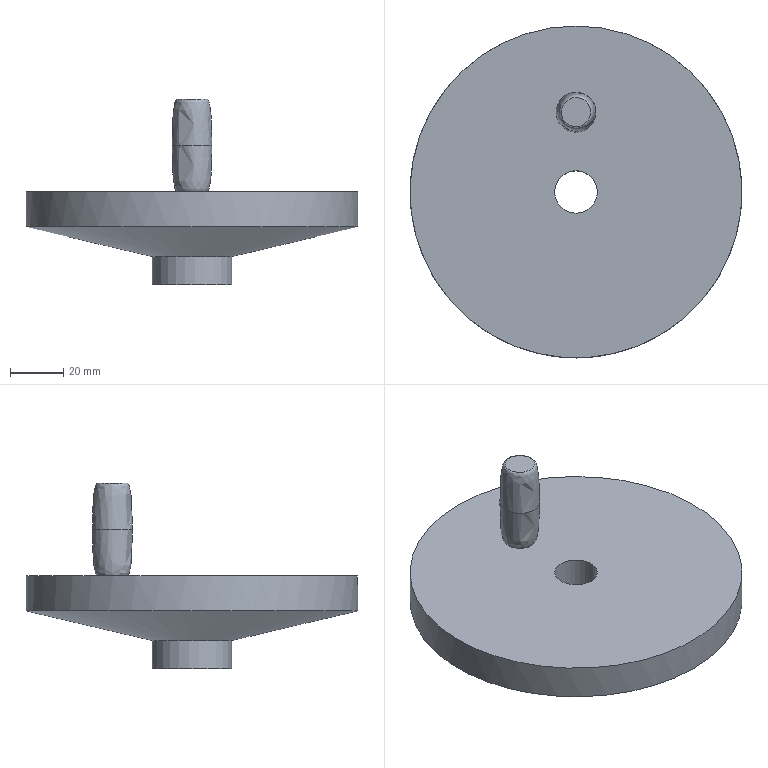Part | STEP file | YBQDJ-YL-10 | 1 solid | 9 faces | box 125 x 125 x 70 mm | volume 226936 mm3 | cylinder 3 | plane 3 | spline 2 | cone 1 | commonest cylinder face diameters 16 x1 30 x1 125 x1
STEP:
#1=CARTESIAN_POINT('',(0.,0.,0.));
#2=DIRECTION('',(0.,0.,1.));
#3=DIRECTION('',(1.,0.,0.));
#4=AXIS2_PLACEMENT_3D('',#1,#2,#3);
#5=CARTESIAN_POINT('',(306.5,-187.,261.));
#6=VERTEX_POINT('',#5);
#7=CARTESIAN_POINT('',(306.5,-195.,261.));
#8=DIRECTION('',(0.,0.,-1.));
#9=DIRECTION('',(0.,1.,0.));
#10=AXIS2_PLACEMENT_3D('',#7,#8,#9);
#11=CIRCLE('',#10,8.);
#12=CARTESIAN_POINT('',(306.5,-195.,-163.));
#13=DIRECTION('',(0.,0.,1.));
#14=DIRECTION('',(0.,-1.,0.));
#15=AXIS2_PLACEMENT_3D('',#12,#13,#14);
#16=CYLINDRICAL_SURFACE('',#15,8.);
#17=CARTESIAN_POINT('',(9.425,424.));
#18=DIRECTION('',(-1.,0.));
#19=VECTOR('',#18,1.);
#20=LINE('',#17,#19);
#21=(GEOMETRIC_REPRESENTATION_CONTEXT(2)PARAMETRIC_REPRESENTATION_CONTEXT()REPRESENTATION_CONTEXT('',''));
#22=DEFINITIONAL_REPRESENTATION('',(#20),#21);
#23=PCURVE('',#16,#22);
#24=CARTESIAN_POINT('',(306.5,-195.,261.));
#25=DIRECTION('',(0.,0.,-1.));
#26=DIRECTION('',(0.,1.,0.));
#27=AXIS2_PLACEMENT_3D('',#24,#25,#26);
#28=PLANE('',#27);
#29=CARTESIAN_POINT('',(0.,0.));
#30=DIRECTION('',(1.,0.));
#31=AXIS2_PLACEMENT_2D('',#29,#30);
#32=CIRCLE('',#31,8.);
#33=(GEOMETRIC_REPRESENTATION_CONTEXT(2)PARAMETRIC_REPRESENTATION_CONTEXT()REPRESENTATION_CONTEXT('',''));
#34=DEFINITIONAL_REPRESENTATION('',(#32),#33);
#35=PCURVE('',#28,#34);
#36=SURFACE_CURVE('',#11,(#23,#35),.PCURVE_S1.);
#37=EDGE_CURVE('',#6,#6,#36,.T.);
#38=ORIENTED_EDGE('',*,*,#37,.T.);
#39=CARTESIAN_POINT('',(306.5,-187.,226.));
#40=VERTEX_POINT('',#39);
#41=CARTESIAN_POINT('',(306.5,-187.,226.));
#42=CARTESIAN_POINT('',(306.5,-187.,261.));
#43=B_SPLINE_CURVE_WITH_KNOTS('',1,(#41,#42),.UNSPECIFIED.,.F.,.F.,(2,2),(389.,424.),.PIECEWISE_BEZIER_KNOTS.);
#44=CARTESIAN_POINT('',(3.142,0.));
#45=DIRECTION('',(0.,1.));
#46=VECTOR('',#45,1.);
#47=LINE('',#44,#46);
#48=(GEOMETRIC_REPRESENTATION_CONTEXT(2)PARAMETRIC_REPRESENTATION_CONTEXT()REPRESENTATION_CONTEXT('',''));
#49=DEFINITIONAL_REPRESENTATION('',(#47),#48);
#50=PCURVE('',#16,#49);
#51=CARTESIAN_POINT('',(9.425,0.));
#52=DIRECTION('',(0.,1.));
#53=VECTOR('',#52,1.);
#54=LINE('',#51,#53);
#55=(GEOMETRIC_REPRESENTATION_CONTEXT(2)PARAMETRIC_REPRESENTATION_CONTEXT()REPRESENTATION_CONTEXT('',''));
#56=DEFINITIONAL_REPRESENTATION('',(#54),#55);
#57=PCURVE('',#16,#56);
#58=SEAM_CURVE('',#43,(#50,#57),.PCURVE_S1.);
#59=EDGE_CURVE('',#40,#6,#58,.T.);
#60=ORIENTED_EDGE('',*,*,#59,.F.);
#61=CARTESIAN_POINT('',(306.5,-195.,226.));
#62=DIRECTION('',(0.,0.,-1.));
#63=DIRECTION('',(0.,1.,0.));
#64=AXIS2_PLACEMENT_3D('',#61,#62,#63);
#65=CIRCLE('',#64,8.);
#66=CARTESIAN_POINT('',(9.425,389.));
#67=DIRECTION('',(-1.,0.));
#68=VECTOR('',#67,1.);
#69=LINE('',#66,#68);
#70=(GEOMETRIC_REPRESENTATION_CONTEXT(2)PARAMETRIC_REPRESENTATION_CONTEXT()REPRESENTATION_CONTEXT('',''));
#71=DEFINITIONAL_REPRESENTATION('',(#69),#70);
#72=PCURVE('',#16,#71);
#73=CARTESIAN_POINT('',(306.5,-181.,226.));
#74=DIRECTION('',(0.,0.,-1.));
#75=DIRECTION('',(0.,1.,0.));
#76=AXIS2_PLACEMENT_3D('',#73,#74,#75);
#77=PLANE('',#76);
#78=CARTESIAN_POINT('',(-14.,0.));
#79=DIRECTION('',(1.,0.));
#80=AXIS2_PLACEMENT_2D('',#78,#79);
#81=CIRCLE('',#80,8.);
#82=(GEOMETRIC_REPRESENTATION_CONTEXT(2)PARAMETRIC_REPRESENTATION_CONTEXT()REPRESENTATION_CONTEXT('',''));
#83=DEFINITIONAL_REPRESENTATION('',(#81),#82);
#84=PCURVE('',#77,#83);
#85=SURFACE_CURVE('',#65,(#72,#84),.PCURVE_S1.);
#86=EDGE_CURVE('',#40,#40,#85,.T.);
#87=ORIENTED_EDGE('',*,*,#86,.F.);
#88=ORIENTED_EDGE('',*,*,#59,.T.);
#89=EDGE_LOOP('',(#38,#60,#87,#88));
#90=FACE_BOUND('',#89,.F.);
#91=ADVANCED_FACE('',(#90),#16,.F.);
#92=CARTESIAN_POINT('',(301.,-165.,296.));
#93=VERTEX_POINT('',#92);
#94=CARTESIAN_POINT('',(301.,-165.,296.));
#95=CARTESIAN_POINT('',(301.,-166.441,296.));
#96=CARTESIAN_POINT('',(301.594,-167.872,296.));
#97=CARTESIAN_POINT('',(302.611,-168.889,296.));
#98=CARTESIAN_POINT('',(303.628,-169.906,296.));
#99=CARTESIAN_POINT('',(305.062,-170.5,296.));
#100=CARTESIAN_POINT('',(306.5,-170.5,296.));
#101=CARTESIAN_POINT('',(307.938,-170.5,296.));
#102=CARTESIAN_POINT('',(309.372,-169.906,296.));
#103=CARTESIAN_POINT('',(310.389,-168.889,296.));
#104=CARTESIAN_POINT('',(311.406,-167.872,296.));
#105=CARTESIAN_POINT('',(312.,-166.438,296.));
#106=CARTESIAN_POINT('',(312.,-165.,296.));
#107=CARTESIAN_POINT('',(312.,-163.562,296.));
#108=CARTESIAN_POINT('',(311.406,-162.128,296.));
#109=CARTESIAN_POINT('',(310.389,-161.111,296.));
#110=CARTESIAN_POINT('',(309.372,-160.094,296.));
#111=CARTESIAN_POINT('',(307.938,-159.5,296.));
#112=CARTESIAN_POINT('',(306.5,-159.5,296.));
#113=CARTESIAN_POINT('',(305.062,-159.5,296.));
#114=CARTESIAN_POINT('',(303.628,-160.094,296.));
#115=CARTESIAN_POINT('',(302.611,-161.111,296.));
#116=CARTESIAN_POINT('',(301.594,-162.128,296.));
#117=CARTESIAN_POINT('',(301.,-163.561,296.));
#118=CARTESIAN_POINT('',(301.,-165.,296.));
#119=B_SPLINE_CURVE_WITH_KNOTS('',3,(#94,#95,#96,#97,#98,#99,#100,#101,#102,#103,#104,#105,#106,#107,#108,#109,#110,#111,#112,#113,#114,#115,#116,#117,#118),.UNSPECIFIED.,.T.,.F.,(1,3,3,3,3,3,3,3,3,3,1),(-0.125,0.,0.125,0.25,0.375,0.5,0.625,0.75,0.875,1.,1.125),.UNSPECIFIED.);
#120=CARTESIAN_POINT('',(306.5,-165.,296.));
#121=DIRECTION('',(0.,0.,-1.));
#122=DIRECTION('',(0.,-1.,0.));
#123=AXIS2_PLACEMENT_3D('',#120,#121,#122);
#124=PLANE('',#123);
#125=CARTESIAN_POINT('',(0.,5.5));
#126=CARTESIAN_POINT('',(1.441,5.5));
#127=CARTESIAN_POINT('',(2.872,4.906));
#128=CARTESIAN_POINT('',(3.889,3.889));
#129=CARTESIAN_POINT('',(4.906,2.872));
#130=CARTESIAN_POINT('',(5.5,1.438));
#131=CARTESIAN_POINT('',(5.5,0.));
#132=CARTESIAN_POINT('',(5.5,-1.438));
#133=CARTESIAN_POINT('',(4.906,-2.872));
#134=CARTESIAN_POINT('',(3.889,-3.889));
#135=CARTESIAN_POINT('',(2.872,-4.906));
#136=CARTESIAN_POINT('',(1.438,-5.5));
#137=CARTESIAN_POINT('',(0.,-5.5));
#138=CARTESIAN_POINT('',(-1.438,-5.5));
#139=CARTESIAN_POINT('',(-2.872,-4.906));
#140=CARTESIAN_POINT('',(-3.889,-3.889));
#141=CARTESIAN_POINT('',(-4.906,-2.872));
#142=CARTESIAN_POINT('',(-5.5,-1.438));
#143=CARTESIAN_POINT('',(-5.5,0.));
#144=CARTESIAN_POINT('',(-5.5,1.438));
#145=CARTESIAN_POINT('',(-4.906,2.872));
#146=CARTESIAN_POINT('',(-3.889,3.889));
#147=CARTESIAN_POINT('',(-2.872,4.906));
#148=CARTESIAN_POINT('',(-1.439,5.5));
#149=CARTESIAN_POINT('',(0.,5.5));
#150=B_SPLINE_CURVE_WITH_KNOTS('',3,(#125,#126,#127,#128,#129,#130,#131,#132,#133,#134,#135,#136,#137,#138,#139,#140,#141,#142,#143,#144,#145,#146,#147,#148,#149),.UNSPECIFIED.,.T.,.F.,(1,3,3,3,3,3,3,3,3,3,1),(-0.125,0.,0.125,0.25,0.375,0.5,0.625,0.75,0.875,1.,1.125),.UNSPECIFIED.);
#151=(GEOMETRIC_REPRESENTATION_CONTEXT(2)PARAMETRIC_REPRESENTATION_CONTEXT()REPRESENTATION_CONTEXT('',''));
#152=DEFINITIONAL_REPRESENTATION('',(#150),#151);
#153=PCURVE('',#124,#152);
#154=CARTESIAN_POINT('',(299.,-165.,278.5));
#155=CARTESIAN_POINT('',(299.,-165.982,278.5));
#156=CARTESIAN_POINT('',(299.195,-166.963,278.5));
#157=CARTESIAN_POINT('',(299.947,-168.777,278.5));
#158=CARTESIAN_POINT('',(300.502,-169.609,278.5));
#159=CARTESIAN_POINT('',(301.891,-170.998,278.5));
#160=CARTESIAN_POINT('',(302.723,-171.553,278.5));
#161=CARTESIAN_POINT('',(304.537,-172.305,278.5));
#162=CARTESIAN_POINT('',(305.518,-172.5,278.5));
#163=CARTESIAN_POINT('',(307.482,-172.5,278.5));
#164=CARTESIAN_POINT('',(308.463,-172.305,278.5));
#165=CARTESIAN_POINT('',(310.277,-171.553,278.5));
#166=CARTESIAN_POINT('',(311.109,-170.998,278.5));
#167=CARTESIAN_POINT('',(312.498,-169.609,278.5));
#168=CARTESIAN_POINT('',(313.053,-168.777,278.5));
#169=CARTESIAN_POINT('',(313.805,-166.963,278.5));
#170=CARTESIAN_POINT('',(314.,-165.982,278.5));
#171=CARTESIAN_POINT('',(314.,-164.018,278.5));
#172=CARTESIAN_POINT('',(313.805,-163.037,278.5));
#173=CARTESIAN_POINT('',(313.053,-161.223,278.5));
#174=CARTESIAN_POINT('',(312.498,-160.391,278.5));
#175=CARTESIAN_POINT('',(311.109,-159.002,278.5));
#176=CARTESIAN_POINT('',(310.277,-158.447,278.5));
#177=CARTESIAN_POINT('',(308.463,-157.695,278.5));
#178=CARTESIAN_POINT('',(307.482,-157.5,278.5));
#179=CARTESIAN_POINT('',(305.518,-157.5,278.5));
#180=CARTESIAN_POINT('',(304.537,-157.695,278.5));
#181=CARTESIAN_POINT('',(302.723,-158.447,278.5));
#182=CARTESIAN_POINT('',(301.891,-159.002,278.5));
#183=CARTESIAN_POINT('',(300.502,-160.391,278.5));
#184=CARTESIAN_POINT('',(299.947,-161.223,278.5));
#185=CARTESIAN_POINT('',(299.195,-163.037,278.5));
#186=CARTESIAN_POINT('',(299.,-164.018,278.5));
#187=CARTESIAN_POINT('',(299.,-165.,278.5));
#188=CARTESIAN_POINT('',(299.,-165.,296.));
#189=CARTESIAN_POINT('',(299.,-165.982,296.));
#190=CARTESIAN_POINT('',(299.195,-166.963,296.));
#191=CARTESIAN_POINT('',(299.947,-168.777,296.));
#192=CARTESIAN_POINT('',(300.502,-169.609,296.));
#193=CARTESIAN_POINT('',(301.891,-170.998,296.));
#194=CARTESIAN_POINT('',(302.723,-171.553,296.));
#195=CARTESIAN_POINT('',(304.537,-172.305,296.));
#196=CARTESIAN_POINT('',(305.518,-172.5,296.));
#197=CARTESIAN_POINT('',(307.482,-172.5,296.));
#198=CARTESIAN_POINT('',(308.463,-172.305,296.));
#199=CARTESIAN_POINT('',(310.277,-171.553,296.));
#200=CARTESIAN_POINT('',(311.109,-170.998,296.));
#201=CARTESIAN_POINT('',(312.498,-169.609,296.));
#202=CARTESIAN_POINT('',(313.053,-168.777,296.));
#203=CARTESIAN_POINT('',(313.805,-166.963,296.));
#204=CARTESIAN_POINT('',(314.,-165.982,296.));
#205=CARTESIAN_POINT('',(314.,-164.018,296.));
#206=CARTESIAN_POINT('',(313.805,-163.037,296.));
#207=CARTESIAN_POINT('',(313.053,-161.223,296.));
#208=CARTESIAN_POINT('',(312.498,-160.391,296.));
#209=CARTESIAN_POINT('',(311.109,-159.002,296.));
#210=CARTESIAN_POINT('',(310.277,-158.447,296.));
#211=CARTESIAN_POINT('',(308.463,-157.695,296.));
#212=CARTESIAN_POINT('',(307.482,-157.5,296.));
#213=CARTESIAN_POINT('',(305.518,-157.5,296.));
#214=CARTESIAN_POINT('',(304.537,-157.695,296.));
#215=CARTESIAN_POINT('',(302.723,-158.447,296.));
#216=CARTESIAN_POINT('',(301.891,-159.002,296.));
#217=CARTESIAN_POINT('',(300.502,-160.391,296.));
#218=CARTESIAN_POINT('',(299.947,-161.223,296.));
#219=CARTESIAN_POINT('',(299.195,-163.037,296.));
#220=CARTESIAN_POINT('',(299.,-164.018,296.));
#221=CARTESIAN_POINT('',(299.,-165.,296.));
#222=CARTESIAN_POINT('',(301.,-165.,296.));
#223=CARTESIAN_POINT('',(301.,-165.72,296.));
#224=CARTESIAN_POINT('',(301.143,-166.44,296.));
#225=CARTESIAN_POINT('',(301.694,-167.77,296.));
#226=CARTESIAN_POINT('',(302.102,-168.38,296.));
#227=CARTESIAN_POINT('',(303.12,-169.398,296.));
#228=CARTESIAN_POINT('',(303.73,-169.806,296.));
#229=CARTESIAN_POINT('',(305.06,-170.357,296.));
#230=CARTESIAN_POINT('',(305.78,-170.5,296.));
#231=CARTESIAN_POINT('',(307.22,-170.5,296.));
#232=CARTESIAN_POINT('',(307.94,-170.357,296.));
#233=CARTESIAN_POINT('',(309.27,-169.806,296.));
#234=CARTESIAN_POINT('',(309.88,-169.398,296.));
#235=CARTESIAN_POINT('',(310.898,-168.38,296.));
#236=CARTESIAN_POINT('',(311.306,-167.77,296.));
#237=CARTESIAN_POINT('',(311.857,-166.44,296.));
#238=CARTESIAN_POINT('',(312.,-165.72,296.));
#239=CARTESIAN_POINT('',(312.,-164.28,296.));
#240=CARTESIAN_POINT('',(311.857,-163.56,296.));
#241=CARTESIAN_POINT('',(311.306,-162.23,296.));
#242=CARTESIAN_POINT('',(310.898,-161.62,296.));
#243=CARTESIAN_POINT('',(309.88,-160.602,296.));
#244=CARTESIAN_POINT('',(309.27,-160.194,296.));
#245=CARTESIAN_POINT('',(307.94,-159.643,296.));
#246=CARTESIAN_POINT('',(307.22,-159.5,296.));
#247=CARTESIAN_POINT('',(305.78,-159.5,296.));
#248=CARTESIAN_POINT('',(305.06,-159.643,296.));
#249=CARTESIAN_POINT('',(303.73,-160.194,296.));
#250=CARTESIAN_POINT('',(303.12,-160.602,296.));
#251=CARTESIAN_POINT('',(302.102,-161.62,296.));
#252=CARTESIAN_POINT('',(301.694,-162.23,296.));
#253=CARTESIAN_POINT('',(301.143,-163.56,296.));
#254=CARTESIAN_POINT('',(301.,-164.28,296.));
#255=CARTESIAN_POINT('',(301.,-165.,296.));
#256=(BOUNDED_SURFACE()B_SPLINE_SURFACE(2,3,((#154,#155,#156,#157,#158,#159,#160,#161,#162,#163,#164,#165,#166,#167,#168,#169,#170,#171,#172,#173,#174,#175,#176,#177,#178,#179,#180,#181,#182,#183,#184,#185,#186,#187),(#188,#189,#190,#191,#192,#193,#194,#195,#196,#197,#198,#199,#200,#201,#202,#203,#204,#205,#206,#207,#208,#209,#210,#211,#212,#213,#214,#215,#216,#217,#218,#219,#220,#221),(#222,#223,#224,#225,#226,#227,#228,#229,#230,#231,#232,#233,#234,#235,#236,#237,#238,#239,#240,#241,#242,#243,#244,#245,#246,#247,#248,#249,#250,#251,#252,#253,#254,#255)),.UNSPECIFIED.,.F.,.T.,.F.)B_SPLINE_SURFACE_WITH_KNOTS((3,3),(1,3,2,2,2,2,2,2,2,2,2,2,2,2,2,2,2,3,1),(0.,1.),(-0.0625,0.,0.0625,0.125,0.1875,0.25,0.3125,0.375,0.4375,0.5,0.5625,0.625,0.6875,0.75,0.8125,0.875,0.9375,1.,1.062),.UNSPECIFIED.)GEOMETRIC_REPRESENTATION_ITEM()RATIONAL_B_SPLINE_SURFACE(((1.,1.,1.,1.,1.,1.,1.,1.,1.,1.,1.,1.,1.,1.,1.,1.,1.,1.,1.,1.,1.,1.,1.,1.,1.,1.,1.,1.,1.,1.,1.,1.,1.,1.),(1.061,1.061,1.061,1.061,1.061,1.061,1.061,1.061,1.061,1.061,1.061,1.061,1.061,1.061,1.061,1.061,1.061,1.061,1.061,1.061,1.061,1.061,1.061,1.061,1.061,1.061,1.061,1.061,1.061,1.061,1.061,1.061,1.061,1.061),(1.,1.,1.,1.,1.,1.,1.,1.,1.,1.,1.,1.,1.,1.,1.,1.,1.,1.,1.,1.,1.,1.,1.,1.,1.,1.,1.,1.,1.,1.,1.,1.,1.,1.)))REPRESENTATION_ITEM('')SURFACE());
#257=CARTESIAN_POINT('',(1.,0.));
#258=DIRECTION('',(0.,1.));
#259=VECTOR('',#258,1.);
#260=LINE('',#257,#259);
#261=(GEOMETRIC_REPRESENTATION_CONTEXT(2)PARAMETRIC_REPRESENTATION_CONTEXT()REPRESENTATION_CONTEXT('',''));
#262=DEFINITIONAL_REPRESENTATION('',(#260),#261);
#263=PCURVE('',#256,#262);
#264=SURFACE_CURVE('',#119,(#153,#263),.PCURVE_S1.);
#265=EDGE_CURVE('',#93,#93,#264,.T.);
#266=ORIENTED_EDGE('',*,*,#265,.T.);
#267=EDGE_LOOP('',(#266));
#268=FACE_BOUND('',#267,.T.);
#269=ADVANCED_FACE('',(#268),#124,.F.);
#270=CARTESIAN_POINT('',(299.,-165.,278.5));
#271=VERTEX_POINT('',#270);
#272=CARTESIAN_POINT('',(299.,-165.,278.5));
#273=CARTESIAN_POINT('',(299.,-165.982,278.5));
#274=CARTESIAN_POINT('',(299.195,-166.963,278.5));
#275=CARTESIAN_POINT('',(299.947,-168.777,278.5));
#276=CARTESIAN_POINT('',(300.502,-169.609,278.5));
#277=CARTESIAN_POINT('',(301.891,-170.998,278.5));
#278=CARTESIAN_POINT('',(302.723,-171.553,278.5));
#279=CARTESIAN_POINT('',(304.537,-172.305,278.5));
#280=CARTESIAN_POINT('',(305.518,-172.5,278.5));
#281=CARTESIAN_POINT('',(307.482,-172.5,278.5));
#282=CARTESIAN_POINT('',(308.463,-172.305,278.5));
#283=CARTESIAN_POINT('',(310.277,-171.553,278.5));
#284=CARTESIAN_POINT('',(311.109,-170.998,278.5));
#285=CARTESIAN_POINT('',(312.498,-169.609,278.5));
#286=CARTESIAN_POINT('',(313.053,-168.777,278.5));
#287=CARTESIAN_POINT('',(313.805,-166.963,278.5));
#288=CARTESIAN_POINT('',(314.,-165.982,278.5));
#289=CARTESIAN_POINT('',(314.,-164.018,278.5));
#290=CARTESIAN_POINT('',(313.805,-163.037,278.5));
#291=CARTESIAN_POINT('',(313.053,-161.223,278.5));
#292=CARTESIAN_POINT('',(312.498,-160.391,278.5));
#293=CARTESIAN_POINT('',(311.109,-159.002,278.5));
#294=CARTESIAN_POINT('',(310.277,-158.447,278.5));
#295=CARTESIAN_POINT('',(308.463,-157.695,278.5));
#296=CARTESIAN_POINT('',(307.482,-157.5,278.5));
#297=CARTESIAN_POINT('',(305.518,-157.5,278.5));
#298=CARTESIAN_POINT('',(304.537,-157.695,278.5));
#299=CARTESIAN_POINT('',(302.723,-158.447,278.5));
#300=CARTESIAN_POINT('',(301.891,-159.002,278.5));
#301=CARTESIAN_POINT('',(300.502,-160.391,278.5));
#302=CARTESIAN_POINT('',(299.947,-161.223,278.5));
#303=CARTESIAN_POINT('',(299.195,-163.037,278.5));
#304=CARTESIAN_POINT('',(299.,-164.018,278.5));
#305=CARTESIAN_POINT('',(299.,-165.,278.5));
#306=B_SPLINE_CURVE_WITH_KNOTS('',3,(#272,#273,#274,#275,#276,#277,#278,#279,#280,#281,#282,#283,#284,#285,#286,#287,#288,#289,#290,#291,#292,#293,#294,#295,#296,#297,#298,#299,#300,#301,#302,#303,#304,#305),.UNSPECIFIED.,.T.,.F.,(1,3,2,2,2,2,2,2,2,2,2,2,2,2,2,2,2,3,1),(-0.0625,0.,0.0625,0.125,0.1875,0.25,0.3125,0.375,0.4375,0.5,0.5625,0.625,0.6875,0.75,0.8125,0.875,0.9375,1.,1.062),.UNSPECIFIED.);
#307=CARTESIAN_POINT('',(0.,0.));
#308=DIRECTION('',(0.,1.));
#309=VECTOR('',#308,1.);
#310=LINE('',#307,#309);
#311=(GEOMETRIC_REPRESENTATION_CONTEXT(2)PARAMETRIC_REPRESENTATION_CONTEXT()REPRESENTATION_CONTEXT('',''));
#312=DEFINITIONAL_REPRESENTATION('',(#310),#311);
#313=PCURVE('',#256,#312);
#314=CARTESIAN_POINT('',(299.,-165.,278.5));
#315=CARTESIAN_POINT('',(299.,-165.982,278.5));
#316=CARTESIAN_POINT('',(299.195,-166.963,278.5));
#317=CARTESIAN_POINT('',(299.947,-168.777,278.5));
#318=CARTESIAN_POINT('',(300.502,-169.609,278.5));
#319=CARTESIAN_POINT('',(301.891,-170.998,278.5));
#320=CARTESIAN_POINT('',(302.723,-171.553,278.5));
#321=CARTESIAN_POINT('',(304.537,-172.305,278.5));
#322=CARTESIAN_POINT('',(305.518,-172.5,278.5));
#323=CARTESIAN_POINT('',(307.482,-172.5,278.5));
#324=CARTESIAN_POINT('',(308.463,-172.305,278.5));
#325=CARTESIAN_POINT('',(310.277,-171.553,278.5));
#326=CARTESIAN_POINT('',(311.109,-170.998,278.5));
#327=CARTESIAN_POINT('',(312.498,-169.609,278.5));
#328=CARTESIAN_POINT('',(313.053,-168.777,278.5));
#329=CARTESIAN_POINT('',(313.805,-166.963,278.5));
#330=CARTESIAN_POINT('',(314.,-165.982,278.5));
#331=CARTESIAN_POINT('',(314.,-164.018,278.5));
#332=CARTESIAN_POINT('',(313.805,-163.037,278.5));
#333=CARTESIAN_POINT('',(313.053,-161.223,278.5));
#334=CARTESIAN_POINT('',(312.498,-160.391,278.5));
#335=CARTESIAN_POINT('',(311.109,-159.002,278.5));
#336=CARTESIAN_POINT('',(310.277,-158.447,278.5));
#337=CARTESIAN_POINT('',(308.463,-157.695,278.5));
#338=CARTESIAN_POINT('',(307.482,-157.5,278.5));
#339=CARTESIAN_POINT('',(305.518,-157.5,278.5));
#340=CARTESIAN_POINT('',(304.537,-157.695,278.5));
#341=CARTESIAN_POINT('',(302.723,-158.447,278.5));
#342=CARTESIAN_POINT('',(301.891,-159.002,278.5));
#343=CARTESIAN_POINT('',(300.502,-160.391,278.5));
#344=CARTESIAN_POINT('',(299.947,-161.223,278.5));
#345=CARTESIAN_POINT('',(299.195,-163.037,278.5));
#346=CARTESIAN_POINT('',(299.,-164.018,278.5));
#347=CARTESIAN_POINT('',(299.,-165.,278.5));
#348=CARTESIAN_POINT('',(299.,-165.,261.));
#349=CARTESIAN_POINT('',(299.,-165.982,261.));
#350=CARTESIAN_POINT('',(299.195,-166.963,261.));
#351=CARTESIAN_POINT('',(299.947,-168.777,261.));
#352=CARTESIAN_POINT('',(300.502,-169.609,261.));
#353=CARTESIAN_POINT('',(301.891,-170.998,261.));
#354=CARTESIAN_POINT('',(302.723,-171.553,261.));
#355=CARTESIAN_POINT('',(304.537,-172.305,261.));
#356=CARTESIAN_POINT('',(305.518,-172.5,261.));
#357=CARTESIAN_POINT('',(307.482,-172.5,261.));
#358=CARTESIAN_POINT('',(308.463,-172.305,261.));
#359=CARTESIAN_POINT('',(310.277,-171.553,261.));
#360=CARTESIAN_POINT('',(311.109,-170.998,261.));
#361=CARTESIAN_POINT('',(312.498,-169.609,261.));
#362=CARTESIAN_POINT('',(313.053,-168.777,261.));
#363=CARTESIAN_POINT('',(313.805,-166.963,261.));
#364=CARTESIAN_POINT('',(314.,-165.982,261.));
#365=CARTESIAN_POINT('',(314.,-164.018,261.));
#366=CARTESIAN_POINT('',(313.805,-163.037,261.));
#367=CARTESIAN_POINT('',(313.053,-161.223,261.));
#368=CARTESIAN_POINT('',(312.498,-160.391,261.));
#369=CARTESIAN_POINT('',(311.109,-159.002,261.));
#370=CARTESIAN_POINT('',(310.277,-158.447,261.));
#371=CARTESIAN_POINT('',(308.463,-157.695,261.));
#372=CARTESIAN_POINT('',(307.482,-157.5,261.));
#373=CARTESIAN_POINT('',(305.518,-157.5,261.));
#374=CARTESIAN_POINT('',(304.537,-157.695,261.));
#375=CARTESIAN_POINT('',(302.723,-158.447,261.));
#376=CARTESIAN_POINT('',(301.891,-159.002,261.));
#377=CARTESIAN_POINT('',(300.502,-160.391,261.));
#378=CARTESIAN_POINT('',(299.947,-161.223,261.));
#379=CARTESIAN_POINT('',(299.195,-163.037,261.));
#380=CARTESIAN_POINT('',(299.,-164.018,261.));
#381=CARTESIAN_POINT('',(299.,-165.,261.));
#382=CARTESIAN_POINT('',(301.,-165.,261.));
#383=CARTESIAN_POINT('',(301.,-165.72,261.));
#384=CARTESIAN_POINT('',(301.143,-166.44,261.));
#385=CARTESIAN_POINT('',(301.694,-167.77,261.));
#386=CARTESIAN_POINT('',(302.102,-168.38,261.));
#387=CARTESIAN_POINT('',(303.12,-169.398,261.));
#388=CARTESIAN_POINT('',(303.73,-169.806,261.));
#389=CARTESIAN_POINT('',(305.06,-170.357,261.));
#390=CARTESIAN_POINT('',(305.78,-170.5,261.));
#391=CARTESIAN_POINT('',(307.22,-170.5,261.));
#392=CARTESIAN_POINT('',(307.94,-170.357,261.));
#393=CARTESIAN_POINT('',(309.27,-169.806,261.));
#394=CARTESIAN_POINT('',(309.88,-169.398,261.));
#395=CARTESIAN_POINT('',(310.898,-168.38,261.));
#396=CARTESIAN_POINT('',(311.306,-167.77,261.));
#397=CARTESIAN_POINT('',(311.857,-166.44,261.));
#398=CARTESIAN_POINT('',(312.,-165.72,261.));
#399=CARTESIAN_POINT('',(312.,-164.28,261.));
#400=CARTESIAN_POINT('',(311.857,-163.56,261.));
#401=CARTESIAN_POINT('',(311.306,-162.23,261.));
#402=CARTESIAN_POINT('',(310.898,-161.62,261.));
#403=CARTESIAN_POINT('',(309.88,-160.602,261.));
#404=CARTESIAN_POINT('',(309.27,-160.194,261.));
#405=CARTESIAN_POINT('',(307.94,-159.643,261.));
#406=CARTESIAN_POINT('',(307.22,-159.5,261.));
#407=CARTESIAN_POINT('',(305.78,-159.5,261.));
#408=CARTESIAN_POINT('',(305.06,-159.643,261.));
#409=CARTESIAN_POINT('',(303.73,-160.194,261.));
#410=CARTESIAN_POINT('',(303.12,-160.602,261.));
#411=CARTESIAN_POINT('',(302.102,-161.62,261.));
#412=CARTESIAN_POINT('',(301.694,-162.23,261.));
#413=CARTESIAN_POINT('',(301.143,-163.56,261.));
#414=CARTESIAN_POINT('',(301.,-164.28,261.));
#415=CARTESIAN_POINT('',(301.,-165.,261.));
#416=(BOUNDED_SURFACE()B_SPLINE_SURFACE(2,3,((#314,#315,#316,#317,#318,#319,#320,#321,#322,#323,#324,#325,#326,#327,#328,#329,#330,#331,#332,#333,#334,#335,#336,#337,#338,#339,#340,#341,#342,#343,#344,#345,#346,#347),(#348,#349,#350,#351,#352,#353,#354,#355,#356,#357,#358,#359,#360,#361,#362,#363,#364,#365,#366,#367,#368,#369,#370,#371,#372,#373,#374,#375,#376,#377,#378,#379,#380,#381),(#382,#383,#384,#385,#386,#387,#388,#389,#390,#391,#392,#393,#394,#395,#396,#397,#398,#399,#400,#401,#402,#403,#404,#405,#406,#407,#408,#409,#410,#411,#412,#413,#414,#415)),.UNSPECIFIED.,.F.,.T.,.F.)B_SPLINE_SURFACE_WITH_KNOTS((3,3),(1,3,2,2,2,2,2,2,2,2,2,2,2,2,2,2,2,3,1),(0.,1.),(-0.0625,0.,0.0625,0.125,0.1875,0.25,0.3125,0.375,0.4375,0.5,0.5625,0.625,0.6875,0.75,0.8125,0.875,0.9375,1.,1.062),.UNSPECIFIED.)GEOMETRIC_REPRESENTATION_ITEM()RATIONAL_B_SPLINE_SURFACE(((1.,1.,1.,1.,1.,1.,1.,1.,1.,1.,1.,1.,1.,1.,1.,1.,1.,1.,1.,1.,1.,1.,1.,1.,1.,1.,1.,1.,1.,1.,1.,1.,1.,1.),(1.061,1.061,1.061,1.061,1.061,1.061,1.061,1.061,1.061,1.061,1.061,1.061,1.061,1.061,1.061,1.061,1.061,1.061,1.061,1.061,1.061,1.061,1.061,1.061,1.061,1.061,1.061,1.061,1.061,1.061,1.061,1.061,1.061,1.061),(1.,1.,1.,1.,1.,1.,1.,1.,1.,1.,1.,1.,1.,1.,1.,1.,1.,1.,1.,1.,1.,1.,1.,1.,1.,1.,1.,1.,1.,1.,1.,1.,1.,1.)))REPRESENTATION_ITEM('')SURFACE());
#417=CARTESIAN_POINT('',(0.,0.));
#418=DIRECTION('',(0.,1.));
#419=VECTOR('',#418,1.);
#420=LINE('',#417,#419);
#421=(GEOMETRIC_REPRESENTATION_CONTEXT(2)PARAMETRIC_REPRESENTATION_CONTEXT()REPRESENTATION_CONTEXT('',''));
#422=DEFINITIONAL_REPRESENTATION('',(#420),#421);
#423=PCURVE('',#416,#422);
#424=SURFACE_CURVE('',#306,(#313,#423),.PCURVE_S1.);
#425=EDGE_CURVE('',#271,#271,#424,.T.);
#426=ORIENTED_EDGE('',*,*,#425,.F.);
#427=CARTESIAN_POINT('',(299.,-165.,278.5));
#428=CARTESIAN_POINT('',(299.,-165.,296.));
#429=CARTESIAN_POINT('',(301.,-165.,296.));
#430=(BOUNDED_CURVE()B_SPLINE_CURVE(2,(#427,#428,#429),.UNSPECIFIED.,.F.,.F.)B_SPLINE_CURVE_WITH_KNOTS((3,3),(0.,1.),.PIECEWISE_BEZIER_KNOTS.)CURVE()GEOMETRIC_REPRESENTATION_ITEM()RATIONAL_B_SPLINE_CURVE((1.,1.061,1.))REPRESENTATION_ITEM(''));
#431=CARTESIAN_POINT('',(0.,0.));
#432=DIRECTION('',(1.,0.));
#433=VECTOR('',#432,1.);
#434=LINE('',#431,#433);
#435=(GEOMETRIC_REPRESENTATION_CONTEXT(2)PARAMETRIC_REPRESENTATION_CONTEXT()REPRESENTATION_CONTEXT('',''));
#436=DEFINITIONAL_REPRESENTATION('',(#434),#435);
#437=PCURVE('',#256,#436);
#438=CARTESIAN_POINT('',(0.,1.));
#439=DIRECTION('',(1.,0.));
#440=VECTOR('',#439,1.);
#441=LINE('',#438,#440);
#442=(GEOMETRIC_REPRESENTATION_CONTEXT(2)PARAMETRIC_REPRESENTATION_CONTEXT()REPRESENTATION_CONTEXT('',''));
#443=DEFINITIONAL_REPRESENTATION('',(#441),#442);
#444=PCURVE('',#256,#443);
#445=SEAM_CURVE('',#430,(#437,#444),.PCURVE_S1.);
#446=EDGE_CURVE('',#271,#93,#445,.T.);
#447=ORIENTED_EDGE('',*,*,#446,.T.);
#448=ORIENTED_EDGE('',*,*,#265,.T.);
#449=ORIENTED_EDGE('',*,*,#446,.F.);
#450=EDGE_LOOP('',(#426,#447,#448,#449));
#451=FACE_BOUND('',#450,.F.);
#452=ADVANCED_FACE('',(#451),#256,.F.);
#453=ORIENTED_EDGE('',*,*,#425,.F.);
#454=CARTESIAN_POINT('',(301.,-165.,261.));
#455=VERTEX_POINT('',#454);
#456=CARTESIAN_POINT('',(299.,-165.,278.5));
#457=CARTESIAN_POINT('',(299.,-165.,261.));
#458=CARTESIAN_POINT('',(301.,-165.,261.));
#459=(BOUNDED_CURVE()B_SPLINE_CURVE(2,(#456,#457,#458),.UNSPECIFIED.,.F.,.F.)B_SPLINE_CURVE_WITH_KNOTS((3,3),(0.,1.),.PIECEWISE_BEZIER_KNOTS.)CURVE()GEOMETRIC_REPRESENTATION_ITEM()RATIONAL_B_SPLINE_CURVE((1.,1.061,1.))REPRESENTATION_ITEM(''));
#460=CARTESIAN_POINT('',(0.,0.));
#461=DIRECTION('',(1.,0.));
#462=VECTOR('',#461,1.);
#463=LINE('',#460,#462);
#464=(GEOMETRIC_REPRESENTATION_CONTEXT(2)PARAMETRIC_REPRESENTATION_CONTEXT()REPRESENTATION_CONTEXT('',''));
#465=DEFINITIONAL_REPRESENTATION('',(#463),#464);
#466=PCURVE('',#416,#465);
#467=CARTESIAN_POINT('',(0.,1.));
#468=DIRECTION('',(1.,0.));
#469=VECTOR('',#468,1.);
#470=LINE('',#467,#469);
#471=(GEOMETRIC_REPRESENTATION_CONTEXT(2)PARAMETRIC_REPRESENTATION_CONTEXT()REPRESENTATION_CONTEXT('',''));
#472=DEFINITIONAL_REPRESENTATION('',(#470),#471);
#473=PCURVE('',#416,#472);
#474=SEAM_CURVE('',#459,(#466,#473),.PCURVE_S1.);
#475=EDGE_CURVE('',#271,#455,#474,.T.);
#476=ORIENTED_EDGE('',*,*,#475,.T.);
#477=CARTESIAN_POINT('',(301.,-165.,261.));
#478=CARTESIAN_POINT('',(301.,-163.561,261.));
#479=CARTESIAN_POINT('',(301.595,-162.127,261.));
#480=CARTESIAN_POINT('',(302.611,-161.111,261.));
#481=CARTESIAN_POINT('',(303.627,-160.095,261.));
#482=CARTESIAN_POINT('',(305.063,-159.5,261.));
#483=CARTESIAN_POINT('',(306.5,-159.5,261.));
#484=CARTESIAN_POINT('',(307.937,-159.5,261.));
#485=CARTESIAN_POINT('',(309.373,-160.095,261.));
#486=CARTESIAN_POINT('',(310.389,-161.111,261.));
#487=CARTESIAN_POINT('',(311.405,-162.127,261.));
#488=CARTESIAN_POINT('',(312.,-163.563,261.));
#489=CARTESIAN_POINT('',(312.,-165.,261.));
#490=CARTESIAN_POINT('',(312.,-166.437,261.));
#491=CARTESIAN_POINT('',(311.405,-167.873,261.));
#492=CARTESIAN_POINT('',(310.389,-168.889,261.));
#493=CARTESIAN_POINT('',(309.373,-169.905,261.));
#494=CARTESIAN_POINT('',(307.937,-170.5,261.));
#495=CARTESIAN_POINT('',(306.5,-170.5,261.));
#496=CARTESIAN_POINT('',(305.063,-170.5,261.));
#497=CARTESIAN_POINT('',(303.627,-169.905,261.));
#498=CARTESIAN_POINT('',(302.611,-168.889,261.));
#499=CARTESIAN_POINT('',(301.595,-167.873,261.));
#500=CARTESIAN_POINT('',(301.,-166.441,261.));
#501=CARTESIAN_POINT('',(301.,-165.,261.));
#502=B_SPLINE_CURVE_WITH_KNOTS('',3,(#477,#478,#479,#480,#481,#482,#483,#484,#485,#486,#487,#488,#489,#490,#491,#492,#493,#494,#495,#496,#497,#498,#499,#500,#501),.UNSPECIFIED.,.T.,.F.,(1,3,3,3,3,3,3,3,3,3,1),(-0.125,0.,0.125,0.25,0.375,0.5,0.625,0.75,0.875,1.,1.125),.UNSPECIFIED.);
#503=CARTESIAN_POINT('',(1.,1.));
#504=DIRECTION('',(0.,-1.));
#505=VECTOR('',#504,1.);
#506=LINE('',#503,#505);
#507=(GEOMETRIC_REPRESENTATION_CONTEXT(2)PARAMETRIC_REPRESENTATION_CONTEXT()REPRESENTATION_CONTEXT('',''));
#508=DEFINITIONAL_REPRESENTATION('',(#506),#507);
#509=PCURVE('',#416,#508);
#510=CARTESIAN_POINT('',(30.,-5.5));
#511=CARTESIAN_POINT('',(31.439,-5.5));
#512=CARTESIAN_POINT('',(32.873,-4.905));
#513=CARTESIAN_POINT('',(33.889,-3.889));
#514=CARTESIAN_POINT('',(34.905,-2.873));
#515=CARTESIAN_POINT('',(35.5,-1.437));
#516=CARTESIAN_POINT('',(35.5,0.));
#517=CARTESIAN_POINT('',(35.5,1.437));
#518=CARTESIAN_POINT('',(34.905,2.873));
#519=CARTESIAN_POINT('',(33.889,3.889));
#520=CARTESIAN_POINT('',(32.873,4.905));
#521=CARTESIAN_POINT('',(31.437,5.5));
#522=CARTESIAN_POINT('',(30.,5.5));
#523=CARTESIAN_POINT('',(28.563,5.5));
#524=CARTESIAN_POINT('',(27.127,4.905));
#525=CARTESIAN_POINT('',(26.111,3.889));
#526=CARTESIAN_POINT('',(25.095,2.873));
#527=CARTESIAN_POINT('',(24.5,1.437));
#528=CARTESIAN_POINT('',(24.5,0.));
#529=CARTESIAN_POINT('',(24.5,-1.437));
#530=CARTESIAN_POINT('',(25.095,-2.873));
#531=CARTESIAN_POINT('',(26.111,-3.889));
#532=CARTESIAN_POINT('',(27.127,-4.905));
#533=CARTESIAN_POINT('',(28.559,-5.5));
#534=CARTESIAN_POINT('',(30.,-5.5));
#535=B_SPLINE_CURVE_WITH_KNOTS('',3,(#510,#511,#512,#513,#514,#515,#516,#517,#518,#519,#520,#521,#522,#523,#524,#525,#526,#527,#528,#529,#530,#531,#532,#533,#534),.UNSPECIFIED.,.T.,.F.,(1,3,3,3,3,3,3,3,3,3,1),(-0.125,0.,0.125,0.25,0.375,0.5,0.625,0.75,0.875,1.,1.125),.UNSPECIFIED.);
#536=(GEOMETRIC_REPRESENTATION_CONTEXT(2)PARAMETRIC_REPRESENTATION_CONTEXT()REPRESENTATION_CONTEXT('',''));
#537=DEFINITIONAL_REPRESENTATION('',(#535),#536);
#538=PCURVE('',#28,#537);
#539=SURFACE_CURVE('',#502,(#509,#538),.PCURVE_S1.);
#540=EDGE_CURVE('',#455,#455,#539,.T.);
#541=ORIENTED_EDGE('',*,*,#540,.F.);
#542=ORIENTED_EDGE('',*,*,#475,.F.);
#543=EDGE_LOOP('',(#453,#476,#541,#542));
#544=FACE_BOUND('',#543,.T.);
#545=ADVANCED_FACE('',(#544),#416,.T.);
#546=CARTESIAN_POINT('',(306.5,-132.5,261.));
#547=VERTEX_POINT('',#546);
#548=CARTESIAN_POINT('',(306.5,-195.,261.));
#549=DIRECTION('',(0.,0.,-1.));
#550=DIRECTION('',(0.,1.,0.));
#551=AXIS2_PLACEMENT_3D('',#548,#549,#550);
#552=CIRCLE('',#551,62.5);
#553=CARTESIAN_POINT('',(0.,0.));
#554=DIRECTION('',(1.,0.));
#555=AXIS2_PLACEMENT_2D('',#553,#554);
#556=CIRCLE('',#555,62.5);
#557=(GEOMETRIC_REPRESENTATION_CONTEXT(2)PARAMETRIC_REPRESENTATION_CONTEXT()REPRESENTATION_CONTEXT('',''));
#558=DEFINITIONAL_REPRESENTATION('',(#556),#557);
#559=PCURVE('',#28,#558);
#560=CARTESIAN_POINT('',(306.5,-195.,261.));
#561=DIRECTION('',(0.,0.,-1.));
#562=DIRECTION('',(0.,1.,0.));
#563=AXIS2_PLACEMENT_3D('',#560,#561,#562);
#564=CYLINDRICAL_SURFACE('',#563,62.5);
#565=CARTESIAN_POINT('',(0.,0.));
#566=DIRECTION('',(1.,0.));
#567=VECTOR('',#566,1.);
#568=LINE('',#565,#567);
#569=(GEOMETRIC_REPRESENTATION_CONTEXT(2)PARAMETRIC_REPRESENTATION_CONTEXT()REPRESENTATION_CONTEXT('',''));
#570=DEFINITIONAL_REPRESENTATION('',(#568),#569);
#571=PCURVE('',#564,#570);
#572=SURFACE_CURVE('',#552,(#559,#571),.PCURVE_S1.);
#573=EDGE_CURVE('',#547,#547,#572,.T.);
#574=ORIENTED_EDGE('',*,*,#573,.F.);
#575=EDGE_LOOP('',(#574));
#576=FACE_BOUND('',#575,.T.);
#577=ORIENTED_EDGE('',*,*,#37,.T.);
#578=EDGE_LOOP('',(#577));
#579=FACE_BOUND('',#578,.T.);
#580=ORIENTED_EDGE('',*,*,#540,.T.);
#581=EDGE_LOOP('',(#580));
#582=FACE_BOUND('',#581,.T.);
#583=ADVANCED_FACE('',(#576,#579,#582),#28,.F.);
#584=CARTESIAN_POINT('',(306.5,-132.5,247.842));
#585=VERTEX_POINT('',#584);
#586=CARTESIAN_POINT('',(306.5,-257.5,247.842));
#587=VERTEX_POINT('',#586);
#588=CARTESIAN_POINT('',(306.5,-195.,247.842));
#589=DIRECTION('',(0.,0.,-1.));
#590=DIRECTION('',(0.,-1.,0.));
#591=AXIS2_PLACEMENT_3D('',#588,#589,#590);
#592=CIRCLE('',#591,62.5);
#593=CARTESIAN_POINT('',(-3.142,13.158));
#594=DIRECTION('',(1.,0.));
#595=VECTOR('',#594,1.);
#596=LINE('',#593,#595);
#597=(GEOMETRIC_REPRESENTATION_CONTEXT(2)PARAMETRIC_REPRESENTATION_CONTEXT()REPRESENTATION_CONTEXT('',''));
#598=DEFINITIONAL_REPRESENTATION('',(#596),#597);
#599=PCURVE('',#564,#598);
#600=CARTESIAN_POINT('',(306.5,-195.,247.842));
#601=DIRECTION('',(0.,0.,1.));
#602=DIRECTION('',(0.,1.,0.));
#603=AXIS2_PLACEMENT_3D('',#600,#601,#602);
#604=CONICAL_SURFACE('',#603,62.5,1.34);
#605=CARTESIAN_POINT('',(9.425,0.));
#606=DIRECTION('',(-1.,0.));
#607=VECTOR('',#606,1.);
#608=LINE('',#605,#607);
#609=(GEOMETRIC_REPRESENTATION_CONTEXT(2)PARAMETRIC_REPRESENTATION_CONTEXT()REPRESENTATION_CONTEXT('',''));
#610=DEFINITIONAL_REPRESENTATION('',(#608),#609);
#611=PCURVE('',#604,#610);
#612=SURFACE_CURVE('',#592,(#599,#611),.PCURVE_S1.);
#613=EDGE_CURVE('',#585,#587,#612,.T.);
#614=ORIENTED_EDGE('',*,*,#613,.F.);
#615=CARTESIAN_POINT('',(306.5,-132.5,261.));
#616=CARTESIAN_POINT('',(306.5,-132.5,247.842));
#617=B_SPLINE_CURVE_WITH_KNOTS('',1,(#615,#616),.UNSPECIFIED.,.F.,.F.,(2,2),(0.,13.158),.PIECEWISE_BEZIER_KNOTS.);
#618=CARTESIAN_POINT('',(0.,0.));
#619=DIRECTION('',(0.,1.));
#620=VECTOR('',#619,1.);
#621=LINE('',#618,#620);
#622=(GEOMETRIC_REPRESENTATION_CONTEXT(2)PARAMETRIC_REPRESENTATION_CONTEXT()REPRESENTATION_CONTEXT('',''));
#623=DEFINITIONAL_REPRESENTATION('',(#621),#622);
#624=PCURVE('',#564,#623);
#625=CARTESIAN_POINT('',(6.283,0.));
#626=DIRECTION('',(0.,1.));
#627=VECTOR('',#626,1.);
#628=LINE('',#625,#627);
#629=(GEOMETRIC_REPRESENTATION_CONTEXT(2)PARAMETRIC_REPRESENTATION_CONTEXT()REPRESENTATION_CONTEXT('',''));
#630=DEFINITIONAL_REPRESENTATION('',(#628),#629);
#631=PCURVE('',#564,#630);
#632=SEAM_CURVE('',#617,(#624,#631),.PCURVE_S1.);
#633=EDGE_CURVE('',#547,#585,#632,.T.);
#634=ORIENTED_EDGE('',*,*,#633,.F.);
#635=ORIENTED_EDGE('',*,*,#573,.T.);
#636=ORIENTED_EDGE('',*,*,#633,.T.);
#637=CARTESIAN_POINT('',(306.5,-195.,247.842));
#638=DIRECTION('',(0.,0.,-1.));
#639=DIRECTION('',(0.,-1.,0.));
#640=AXIS2_PLACEMENT_3D('',#637,#638,#639);
#641=CIRCLE('',#640,62.5);
#642=CARTESIAN_POINT('',(3.142,13.158));
#643=DIRECTION('',(1.,0.));
#644=VECTOR('',#643,1.);
#645=LINE('',#642,#644);
#646=(GEOMETRIC_REPRESENTATION_CONTEXT(2)PARAMETRIC_REPRESENTATION_CONTEXT()REPRESENTATION_CONTEXT('',''));
#647=DEFINITIONAL_REPRESENTATION('',(#645),#646);
#648=PCURVE('',#564,#647);
#649=CARTESIAN_POINT('',(3.142,0.));
#650=DIRECTION('',(-1.,0.));
#651=VECTOR('',#650,1.);
#652=LINE('',#649,#651);
#653=(GEOMETRIC_REPRESENTATION_CONTEXT(2)PARAMETRIC_REPRESENTATION_CONTEXT()REPRESENTATION_CONTEXT('',''));
#654=DEFINITIONAL_REPRESENTATION('',(#652),#653);
#655=PCURVE('',#604,#654);
#656=SURFACE_CURVE('',#641,(#648,#655),.PCURVE_S1.);
#657=EDGE_CURVE('',#587,#585,#656,.T.);
#658=ORIENTED_EDGE('',*,*,#657,.F.);
#659=EDGE_LOOP('',(#614,#634,#635,#636,#658));
#660=FACE_BOUND('',#659,.T.);
#661=ADVANCED_FACE('',(#660),#564,.T.);
#662=CARTESIAN_POINT('',(306.5,-180.,226.));
#663=VERTEX_POINT('',#662);
#664=CARTESIAN_POINT('',(321.5,-195.,226.));
#665=VERTEX_POINT('',#664);
#666=CARTESIAN_POINT('',(306.5,-195.,226.));
#667=DIRECTION('',(0.,0.,1.));
#668=DIRECTION('',(0.,1.,0.));
#669=AXIS2_PLACEMENT_3D('',#666,#667,#668);
#670=CIRCLE('',#669,15.);
#671=CARTESIAN_POINT('',(306.5,-195.,227.));
#672=DIRECTION('',(0.,0.,1.));
#673=DIRECTION('',(0.,-1.,0.));
#674=AXIS2_PLACEMENT_3D('',#671,#672,#673);
#675=CYLINDRICAL_SURFACE('',#674,15.);
#676=CARTESIAN_POINT('',(3.142,-1.));
#677=DIRECTION('',(1.,0.));
#678=VECTOR('',#677,1.);
#679=LINE('',#676,#678);
#680=(GEOMETRIC_REPRESENTATION_CONTEXT(2)PARAMETRIC_REPRESENTATION_CONTEXT()REPRESENTATION_CONTEXT('',''));
#681=DEFINITIONAL_REPRESENTATION('',(#679),#680);
#682=PCURVE('',#675,#681);
#683=CARTESIAN_POINT('',(1.,0.));
#684=CARTESIAN_POINT('',(1.,-25.981));
#685=CARTESIAN_POINT('',(-21.5,-12.99));
#686=CARTESIAN_POINT('',(-44.,0.));
#687=CARTESIAN_POINT('',(-21.5,12.99));
#688=CARTESIAN_POINT('',(1.,25.981));
#689=CARTESIAN_POINT('',(1.,0.));
#690=(BOUNDED_CURVE()B_SPLINE_CURVE(2,(#683,#684,#685,#686,#687,#688,#689),.UNSPECIFIED.,.T.,.F.)B_SPLINE_CURVE_WITH_KNOTS((1,2,2,2,2,1),(-2.094,0.,2.094,4.189,6.283,8.378),.UNSPECIFIED.)CURVE()GEOMETRIC_REPRESENTATION_ITEM()RATIONAL_B_SPLINE_CURVE((1.,0.5,1.,0.5,1.,0.5,1.))REPRESENTATION_ITEM(''));
#691=(GEOMETRIC_REPRESENTATION_CONTEXT(2)PARAMETRIC_REPRESENTATION_CONTEXT()REPRESENTATION_CONTEXT('',''));
#692=DEFINITIONAL_REPRESENTATION('',(#690),#691);
#693=PCURVE('',#77,#692);
#694=SURFACE_CURVE('',#670,(#682,#693),.PCURVE_S1.);
#695=EDGE_CURVE('',#663,#665,#694,.T.);
#696=ORIENTED_EDGE('',*,*,#695,.T.);
#697=CARTESIAN_POINT('',(321.5,-195.,236.677));
#698=VERTEX_POINT('',#697);
#699=CARTESIAN_POINT('',(321.5,-195.,226.));
#700=CARTESIAN_POINT('',(321.5,-195.,236.677));
#701=B_SPLINE_CURVE_WITH_KNOTS('',1,(#699,#700),.UNSPECIFIED.,.F.,.F.,(2,2),(-1.,9.677),.PIECEWISE_BEZIER_KNOTS.);
#702=CARTESIAN_POINT('',(7.854,0.));
#703=DIRECTION('',(0.,1.));
#704=VECTOR('',#703,1.);
#705=LINE('',#702,#704);
#706=(GEOMETRIC_REPRESENTATION_CONTEXT(2)PARAMETRIC_REPRESENTATION_CONTEXT()REPRESENTATION_CONTEXT('',''));
#707=DEFINITIONAL_REPRESENTATION('',(#705),#706);
#708=PCURVE('',#675,#707);
#709=CARTESIAN_POINT('',(1.571,0.));
#710=DIRECTION('',(0.,1.));
#711=VECTOR('',#710,1.);
#712=LINE('',#709,#711);
#713=(GEOMETRIC_REPRESENTATION_CONTEXT(2)PARAMETRIC_REPRESENTATION_CONTEXT()REPRESENTATION_CONTEXT('',''));
#714=DEFINITIONAL_REPRESENTATION('',(#712),#713);
#715=PCURVE('',#675,#714);
#716=SEAM_CURVE('',#701,(#708,#715),.PCURVE_S1.);
#717=EDGE_CURVE('',#665,#698,#716,.T.);
#718=ORIENTED_EDGE('',*,*,#717,.T.);
#719=CARTESIAN_POINT('',(306.5,-180.,236.677));
#720=VERTEX_POINT('',#719);
#721=CARTESIAN_POINT('',(306.5,-195.,236.677));
#722=DIRECTION('',(0.,0.,-1.));
#723=DIRECTION('',(1.,0.,0.));
#724=AXIS2_PLACEMENT_3D('',#721,#722,#723);
#725=CIRCLE('',#724,15.);
#726=CARTESIAN_POINT('',(7.854,9.677));
#727=DIRECTION('',(-1.,0.));
#728=VECTOR('',#727,1.);
#729=LINE('',#726,#728);
#730=(GEOMETRIC_REPRESENTATION_CONTEXT(2)PARAMETRIC_REPRESENTATION_CONTEXT()REPRESENTATION_CONTEXT('',''));
#731=DEFINITIONAL_REPRESENTATION('',(#729),#730);
#732=PCURVE('',#675,#731);
#733=CARTESIAN_POINT('',(4.712,-11.165));
#734=DIRECTION('',(-1.,0.));
#735=VECTOR('',#734,1.);
#736=LINE('',#733,#735);
#737=(GEOMETRIC_REPRESENTATION_CONTEXT(2)PARAMETRIC_REPRESENTATION_CONTEXT()REPRESENTATION_CONTEXT('',''));
#738=DEFINITIONAL_REPRESENTATION('',(#736),#737);
#739=PCURVE('',#604,#738);
#740=SURFACE_CURVE('',#725,(#732,#739),.PCURVE_S1.);
#741=EDGE_CURVE('',#698,#720,#740,.T.);
#742=ORIENTED_EDGE('',*,*,#741,.T.);
#743=CARTESIAN_POINT('',(306.5,-195.,236.677));
#744=DIRECTION('',(0.,0.,-1.));
#745=DIRECTION('',(1.,0.,0.));
#746=AXIS2_PLACEMENT_3D('',#743,#744,#745);
#747=CIRCLE('',#746,15.);
#748=CARTESIAN_POINT('',(7.854,9.677));
#749=DIRECTION('',(-1.,0.));
#750=VECTOR('',#749,1.);
#751=LINE('',#748,#750);
#752=(GEOMETRIC_REPRESENTATION_CONTEXT(2)PARAMETRIC_REPRESENTATION_CONTEXT()REPRESENTATION_CONTEXT('',''));
#753=DEFINITIONAL_REPRESENTATION('',(#751),#752);
#754=PCURVE('',#675,#753);
#755=CARTESIAN_POINT('',(10.996,-11.165));
#756=DIRECTION('',(-1.,0.));
#757=VECTOR('',#756,1.);
#758=LINE('',#755,#757);
#759=(GEOMETRIC_REPRESENTATION_CONTEXT(2)PARAMETRIC_REPRESENTATION_CONTEXT()REPRESENTATION_CONTEXT('',''));
#760=DEFINITIONAL_REPRESENTATION('',(#758),#759);
#761=PCURVE('',#604,#760);
#762=SURFACE_CURVE('',#747,(#754,#761),.PCURVE_S1.);
#763=EDGE_CURVE('',#720,#698,#762,.T.);
#764=ORIENTED_EDGE('',*,*,#763,.T.);
#765=ORIENTED_EDGE('',*,*,#717,.F.);
#766=CARTESIAN_POINT('',(306.5,-195.,226.));
#767=DIRECTION('',(0.,0.,1.));
#768=DIRECTION('',(0.,1.,0.));
#769=AXIS2_PLACEMENT_3D('',#766,#767,#768);
#770=CIRCLE('',#769,15.);
#771=CARTESIAN_POINT('',(-3.142,-1.));
#772=DIRECTION('',(1.,0.));
#773=VECTOR('',#772,1.);
#774=LINE('',#771,#773);
#775=(GEOMETRIC_REPRESENTATION_CONTEXT(2)PARAMETRIC_REPRESENTATION_CONTEXT()REPRESENTATION_CONTEXT('',''));
#776=DEFINITIONAL_REPRESENTATION('',(#774),#775);
#777=PCURVE('',#675,#776);
#778=CARTESIAN_POINT('',(1.,0.));
#779=CARTESIAN_POINT('',(1.,-25.981));
#780=CARTESIAN_POINT('',(-21.5,-12.99));
#781=CARTESIAN_POINT('',(-44.,0.));
#782=CARTESIAN_POINT('',(-21.5,12.99));
#783=CARTESIAN_POINT('',(1.,25.981));
#784=CARTESIAN_POINT('',(1.,0.));
#785=(BOUNDED_CURVE()B_SPLINE_CURVE(2,(#778,#779,#780,#781,#782,#783,#784),.UNSPECIFIED.,.T.,.F.)B_SPLINE_CURVE_WITH_KNOTS((1,2,2,2,2,1),(-2.094,0.,2.094,4.189,6.283,8.378),.UNSPECIFIED.)CURVE()GEOMETRIC_REPRESENTATION_ITEM()RATIONAL_B_SPLINE_CURVE((1.,0.5,1.,0.5,1.,0.5,1.))REPRESENTATION_ITEM(''));
#786=(GEOMETRIC_REPRESENTATION_CONTEXT(2)PARAMETRIC_REPRESENTATION_CONTEXT()REPRESENTATION_CONTEXT('',''));
#787=DEFINITIONAL_REPRESENTATION('',(#785),#786);
#788=PCURVE('',#77,#787);
#789=SURFACE_CURVE('',#770,(#777,#788),.PCURVE_S1.);
#790=EDGE_CURVE('',#665,#663,#789,.T.);
#791=ORIENTED_EDGE('',*,*,#790,.T.);
#792=EDGE_LOOP('',(#696,#718,#742,#764,#765,#791));
#793=FACE_BOUND('',#792,.T.);
#794=ADVANCED_FACE('',(#793),#675,.T.);
#795=ORIENTED_EDGE('',*,*,#86,.F.);
#796=EDGE_LOOP('',(#795));
#797=FACE_BOUND('',#796,.T.);
#798=ORIENTED_EDGE('',*,*,#695,.F.);
#799=ORIENTED_EDGE('',*,*,#790,.F.);
#800=EDGE_LOOP('',(#798,#799));
#801=FACE_BOUND('',#800,.T.);
#802=ADVANCED_FACE('',(#797,#801),#77,.T.);
#803=ORIENTED_EDGE('',*,*,#657,.T.);
#804=CARTESIAN_POINT('',(306.5,-180.,236.677));
#805=CARTESIAN_POINT('',(306.5,-132.5,247.842));
#806=B_SPLINE_CURVE_WITH_KNOTS('',1,(#804,#805),.UNSPECIFIED.,.F.,.F.,(2,2),(-48.795,0.),.PIECEWISE_BEZIER_KNOTS.);
#807=CARTESIAN_POINT('',(0.,0.));
#808=DIRECTION('',(0.,1.));
#809=VECTOR('',#808,1.);
#810=LINE('',#807,#809);
#811=(GEOMETRIC_REPRESENTATION_CONTEXT(2)PARAMETRIC_REPRESENTATION_CONTEXT()REPRESENTATION_CONTEXT('',''));
#812=DEFINITIONAL_REPRESENTATION('',(#810),#811);
#813=PCURVE('',#604,#812);
#814=CARTESIAN_POINT('',(6.283,0.));
#815=DIRECTION('',(0.,1.));
#816=VECTOR('',#815,1.);
#817=LINE('',#814,#816);
#818=(GEOMETRIC_REPRESENTATION_CONTEXT(2)PARAMETRIC_REPRESENTATION_CONTEXT()REPRESENTATION_CONTEXT('',''));
#819=DEFINITIONAL_REPRESENTATION('',(#817),#818);
#820=PCURVE('',#604,#819);
#821=SEAM_CURVE('',#806,(#813,#820),.PCURVE_S1.);
#822=EDGE_CURVE('',#720,#585,#821,.T.);
#823=ORIENTED_EDGE('',*,*,#822,.F.);
#824=ORIENTED_EDGE('',*,*,#741,.F.);
#825=ORIENTED_EDGE('',*,*,#763,.F.);
#826=ORIENTED_EDGE('',*,*,#822,.T.);
#827=ORIENTED_EDGE('',*,*,#613,.T.);
#828=EDGE_LOOP('',(#803,#823,#824,#825,#826,#827));
#829=FACE_BOUND('',#828,.T.);
#830=ADVANCED_FACE('',(#829),#604,.T.);
#831=CLOSED_SHELL('',(#91,#269,#452,#545,#583,#661,#794,#802,#830));
#832=MANIFOLD_SOLID_BREP('',#831);
#833=(LENGTH_UNIT()NAMED_UNIT(*)SI_UNIT(.MILLI.,.METRE.));
#834=UNCERTAINTY_MEASURE_WITH_UNIT(LENGTH_MEASURE(0.001),#833,'','');
#835=(NAMED_UNIT(*)PLANE_ANGLE_UNIT()SI_UNIT($,.RADIAN.));
#836=(NAMED_UNIT(*)SI_UNIT($,.STERADIAN.)SOLID_ANGLE_UNIT());
#837=(GEOMETRIC_REPRESENTATION_CONTEXT(3)GLOBAL_UNCERTAINTY_ASSIGNED_CONTEXT((#834))GLOBAL_UNIT_ASSIGNED_CONTEXT((#833,#835,#836))REPRESENTATION_CONTEXT('',''));
#838=ADVANCED_BREP_SHAPE_REPRESENTATION('',(#4,#832),#837);